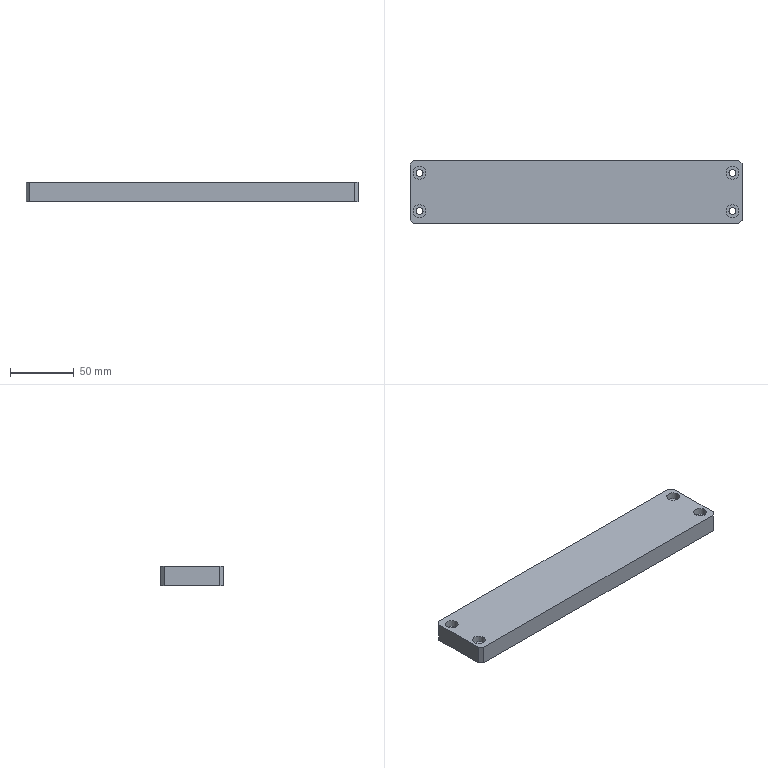CAM job | NX | 3-axis milling, drilling | part box 261 x 50 x 15 mm | stock box 266 x 55 x 20 mm
Tools:
number,name,description,diameter,corner_radius,flute_length,length,flutes
6,D6,平底铣刀-粗,6.0,0.0,25.0,75.0,2
9,D10,平底铣刀-粗,10.0,0.0,35.0,75.0,2
7,D6-J,平底铣刀-精,6.0,0.0,25.0,75.0,2
1,D80R0.8飞刀,圆鼻刀-粗,80.0,0.8,50.0,75.0,2
1,D80R0.8飞刀-J,圆鼻刀-精,80.0,0.8,50.0,75.0,2
2,D6倒角刀,倒角刀,6.0,0.0,3.0,25.0,2
17,ZT5.5,钻头,5.5,0.0,35.0,50.0,2
Operations:
program,operation,operation_type,tool,method,geometry_group,spindle_rpm,surface_speed,feed_per_tooth,feed_cut,feed_plunge,cut_length_mm,path_length_mm,cut_time_min,machine_time_min
B,底壁铣飞面一刀开粗_COPY,VolumeBased25DMillingOperation,D80R0.8飞刀,分层开粗-切深K-步距G,W-B,2800.0,703.696,0.5357,3000.0,100.0,3322.746,6802.966,1.108,1.456
B,底壁铣飞面一刀精光_COPY,VolumeBased25DMillingOperation,D80R0.8飞刀-J,侧刃精光-切深K-步距G,W-B,4000.0,1005.28,0.125,1000.0,100.0,368.998,464.998,0.369,0.3786
B,平面去毛刺6X45L_COPY,SurfaceContour,D6倒角刀,爬面_倒角-切深0-步距G,W-B,6500.0,122.519,0.1154,1500.0,100.0,684.257,1295.504,0.4562,0.5173
A,顶面,FaceMilling,D80R0.8飞刀,侧刃精光-切深K-步距G,W-A,4500.0,1385.0,0.1667,1500.0,100.0,739.333,835.333,0.4929,0.5025
A,外形粗_2,VolumeBased25DMillingOperation,D10,METHOD,W-A,8000.0,251.327,0.375,6000.0,80.0,13588.82,13702.32,2.265,2.276
A,打点,Operation,D6倒角刀,METHOD,W-A,8000.0,150.796,0.1562,2500.0,0.0,10.0,429.035,0.004,0.0459
A,打孔,Operation,ZT5.5,METHOD,W-A,3800.0,65.659,0.1316,1000.0,0.0,74.609,558.254,0.0746,0.123
A,孔粗_1,CylinderMilling,D6,METHOD,W-A,8000.0,150.796,0.125,2000.0,100.0,849.795,1576.195,0.4249,0.4975
A,孔侧_1,CylinderMilling,D6-J,METHOD,W-A,8000.0,150.796,0.0375,600.0,100.0,70.227,819.427,0.117,0.192
A,仅选体,SurfaceContour,D6倒角刀,METHOD,W-A,8000.0,150.796,0.1875,3000.0,100.0,632.272,728.073,0.2108,0.2203
A,铣倒角_1,PlanarMilling,D6倒角刀,METHOD,W-A,8000.0,150.796,0.0375,600.0,100.0,133.995,850.444,0.2233,0.295
A,外形半精_2,VolumeBased25DMillingOperation,D6-J,METHOD,W-A,9000.0,169.646,0.0667,1200.0,100.0,1277.473,1522.993,1.065,1.089